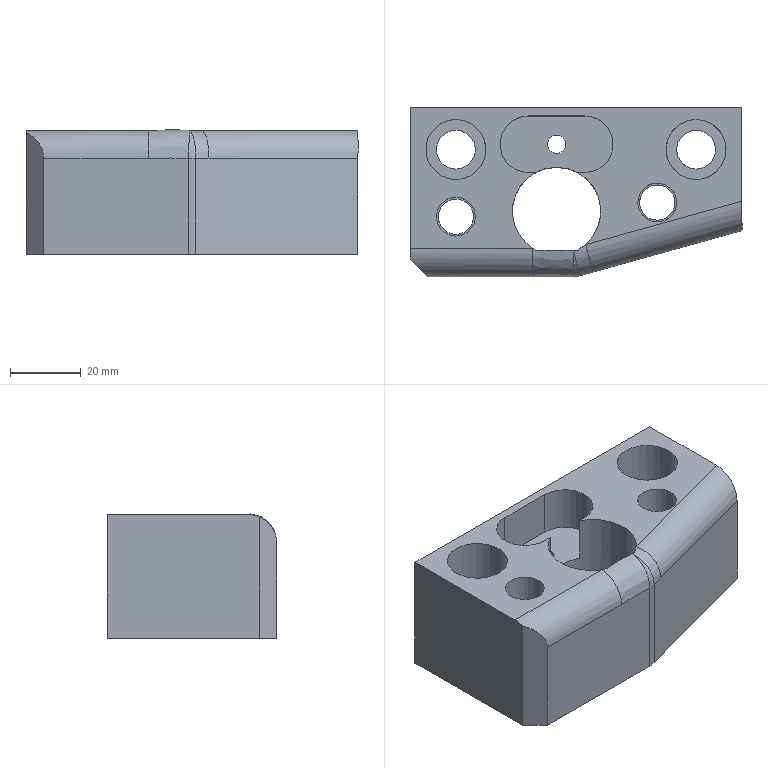Part | STEP file | lll_id4518_x_t | 1 solid | 35 faces | box 94 x 48 x 35.237 mm | volume 104550 mm3 | plane 17 | cylinder 15 | spline 2 | sphere 1 | commonest cylinder face diameters 16 x5 11 x4 10 x2 17 x2 5.206 x1 25 x1
STEP:
#1=CARTESIAN_POINT('',(3581.297,-241.45,-35.));
#2=VERTEX_POINT('',#1);
#3=CARTESIAN_POINT('',(3593.171,-241.45,-35.));
#4=VERTEX_POINT('',#3);
#5=CARTESIAN_POINT('',(3587.234,-230.45,-35.));
#6=DIRECTION('',(0.,0.,-1.));
#7=DIRECTION('',(-1.,0.,0.));
#8=AXIS2_PLACEMENT_3D('',#5,#6,#7);
#9=CIRCLE('',#8,12.5);
#10=EDGE_CURVE('',#2,#4,#9,.T.);
#11=ORIENTED_EDGE('',*,*,#10,.T.);
#12=CARTESIAN_POINT('',(3593.171,-241.45,0.00001673));
#13=VERTEX_POINT('',#12);
#14=CARTESIAN_POINT('',(3593.171,-241.45,-15.));
#15=DIRECTION('',(0.,0.,1.));
#16=VECTOR('',#15,1.);
#17=LINE('',#14,#16);
#18=EDGE_CURVE('',#4,#13,#17,.T.);
#19=ORIENTED_EDGE('',*,*,#18,.T.);
#20=CARTESIAN_POINT('',(3595.413,-239.903,0.00001673));
#21=VERTEX_POINT('',#20);
#22=CARTESIAN_POINT('',(3593.171,-241.45,-0.0001138));
#23=CARTESIAN_POINT('',(3593.485,-241.281,-0.0001498));
#24=CARTESIAN_POINT('',(3593.792,-241.098,-0.0001489));
#25=CARTESIAN_POINT('',(3594.09,-240.902,-0.0001158));
#26=CARTESIAN_POINT('',(3594.552,-240.599,-0.00006449));
#27=CARTESIAN_POINT('',(3594.995,-240.264,0.00001673));
#28=CARTESIAN_POINT('',(3595.413,-239.903,0.00001673));
#29=B_SPLINE_CURVE_WITH_KNOTS('',3,(#22,#23,#24,#25,#26,#27,#28),.UNSPECIFIED.,.F.,.F.,(4,3,4),(0.,0.3921,1.),.UNSPECIFIED.);
#30=EDGE_CURVE('',#13,#21,#29,.T.);
#31=ORIENTED_EDGE('',*,*,#30,.T.);
#32=CARTESIAN_POINT('',(3593.171,-219.45,0.00001673));
#33=VERTEX_POINT('',#32);
#34=CARTESIAN_POINT('',(3587.234,-230.45,0.00001673));
#35=DIRECTION('',(0.,0.,1.));
#36=DIRECTION('',(-1.,0.,0.));
#37=AXIS2_PLACEMENT_3D('',#34,#35,#36);
#38=CIRCLE('',#37,12.5);
#39=EDGE_CURVE('',#21,#33,#38,.T.);
#40=ORIENTED_EDGE('',*,*,#39,.T.);
#41=CARTESIAN_POINT('',(3593.171,-219.45,-13.));
#42=VERTEX_POINT('',#41);
#43=CARTESIAN_POINT('',(3593.171,-219.45,-15.));
#44=DIRECTION('',(0.,0.,1.));
#45=VECTOR('',#44,1.);
#46=LINE('',#43,#45);
#47=EDGE_CURVE('',#42,#33,#46,.T.);
#48=ORIENTED_EDGE('',*,*,#47,.F.);
#49=CARTESIAN_POINT('',(3581.297,-219.45,-13.));
#50=VERTEX_POINT('',#49);
#51=CARTESIAN_POINT('',(3587.234,-230.45,-13.));
#52=DIRECTION('',(0.,0.,1.));
#53=DIRECTION('',(-1.,0.,0.));
#54=AXIS2_PLACEMENT_3D('',#51,#52,#53);
#55=CIRCLE('',#54,12.5);
#56=EDGE_CURVE('',#42,#50,#55,.T.);
#57=ORIENTED_EDGE('',*,*,#56,.T.);
#58=CARTESIAN_POINT('',(3581.297,-219.45,0.00001673));
#59=VERTEX_POINT('',#58);
#60=CARTESIAN_POINT('',(3581.297,-219.45,-15.));
#61=DIRECTION('',(0.,0.,-1.));
#62=VECTOR('',#61,1.);
#63=LINE('',#60,#62);
#64=EDGE_CURVE('',#59,#50,#63,.T.);
#65=ORIENTED_EDGE('',*,*,#64,.F.);
#66=CARTESIAN_POINT('',(3580.452,-240.95,0.00001673));
#67=VERTEX_POINT('',#66);
#68=CARTESIAN_POINT('',(3587.234,-230.45,0.00001673));
#69=DIRECTION('',(0.,0.,1.));
#70=DIRECTION('',(-1.,0.,0.));
#71=AXIS2_PLACEMENT_3D('',#68,#69,#70);
#72=CIRCLE('',#71,12.5);
#73=EDGE_CURVE('',#59,#67,#72,.T.);
#74=ORIENTED_EDGE('',*,*,#73,.T.);
#75=CARTESIAN_POINT('',(3581.297,-241.45,0.00001673));
#76=VERTEX_POINT('',#75);
#77=CARTESIAN_POINT('',(3580.452,-240.95,-0.0008458));
#78=CARTESIAN_POINT('',(3580.727,-241.128,-0.0007971));
#79=CARTESIAN_POINT('',(3581.009,-241.295,-0.0007576));
#80=CARTESIAN_POINT('',(3581.297,-241.45,-0.0007227));
#81=B_SPLINE_CURVE_WITH_KNOTS('',3,(#77,#78,#79,#80),.UNSPECIFIED.,.F.,.F.,(4,4),(0.,1.),.UNSPECIFIED.);
#82=EDGE_CURVE('',#67,#76,#81,.T.);
#83=ORIENTED_EDGE('',*,*,#82,.T.);
#84=CARTESIAN_POINT('',(3581.297,-241.45,-15.));
#85=DIRECTION('',(0.,0.,-1.));
#86=VECTOR('',#85,1.);
#87=LINE('',#84,#86);
#88=EDGE_CURVE('',#76,#2,#87,.T.);
#89=ORIENTED_EDGE('',*,*,#88,.T.);
#90=EDGE_LOOP('',(#11,#19,#31,#40,#48,#57,#65,#74,#83,#89));
#91=FACE_OUTER_BOUND('',#90,.T.);
#92=CARTESIAN_POINT('',(3587.234,-230.45,-15.));
#93=DIRECTION('',(0.,0.,-1.));
#94=DIRECTION('',(1.,0.,0.));
#95=AXIS2_PLACEMENT_3D('',#92,#93,#94);
#96=CYLINDRICAL_SURFACE('',#95,12.5);
#97=ADVANCED_FACE('',(#91),#96,.F.);
#98=CARTESIAN_POINT('',(3618.234,-212.95,0.00001673));
#99=VERTEX_POINT('',#98);
#100=CARTESIAN_POINT('',(3626.734,-212.95,0.00001673));
#101=DIRECTION('',(0.,0.,1.));
#102=DIRECTION('',(-1.,0.,0.));
#103=AXIS2_PLACEMENT_3D('',#100,#101,#102);
#104=CIRCLE('',#103,8.5);
#105=EDGE_CURVE('',#99,#99,#104,.T.);
#106=ORIENTED_EDGE('',*,*,#105,.F.);
#107=EDGE_LOOP('',(#106));
#108=FACE_BOUND('',#107,.T.);
#109=CARTESIAN_POINT('',(3558.734,-226.45,0.00001673));
#110=VERTEX_POINT('',#109);
#111=CARTESIAN_POINT('',(3558.734,-231.95,0.00001673));
#112=DIRECTION('',(0.,0.,1.));
#113=DIRECTION('',(0.,1.,0.));
#114=AXIS2_PLACEMENT_3D('',#111,#112,#113);
#115=CIRCLE('',#114,5.5);
#116=EDGE_CURVE('',#110,#110,#115,.T.);
#117=ORIENTED_EDGE('',*,*,#116,.F.);
#118=EDGE_LOOP('',(#117));
#119=FACE_BOUND('',#118,.T.);
#120=CARTESIAN_POINT('',(3558.734,-221.45,0.00001673));
#121=VERTEX_POINT('',#120);
#122=CARTESIAN_POINT('',(3558.734,-212.95,0.00001673));
#123=DIRECTION('',(0.,0.,-1.));
#124=DIRECTION('',(0.,-1.,0.));
#125=AXIS2_PLACEMENT_3D('',#122,#123,#124);
#126=CIRCLE('',#125,8.5);
#127=EDGE_CURVE('',#121,#121,#126,.T.);
#128=ORIENTED_EDGE('',*,*,#127,.T.);
#129=EDGE_LOOP('',(#128));
#130=FACE_BOUND('',#129,.T.);
#131=CARTESIAN_POINT('',(3610.234,-227.95,0.00001673));
#132=VERTEX_POINT('',#131);
#133=CARTESIAN_POINT('',(3615.734,-227.95,0.00001673));
#134=DIRECTION('',(0.,0.,-1.));
#135=DIRECTION('',(-1.,0.,0.));
#136=AXIS2_PLACEMENT_3D('',#133,#134,#135);
#137=CIRCLE('',#136,5.5);
#138=EDGE_CURVE('',#132,#132,#137,.T.);
#139=ORIENTED_EDGE('',*,*,#138,.T.);
#140=EDGE_LOOP('',(#139));
#141=FACE_BOUND('',#140,.T.);
#142=CARTESIAN_POINT('',(3595.234,-219.45,0.00001673));
#143=VERTEX_POINT('',#142);
#144=CARTESIAN_POINT('',(3595.234,-203.45,0.00001673));
#145=VERTEX_POINT('',#144);
#146=CARTESIAN_POINT('',(3595.234,-211.45,0.00001673));
#147=DIRECTION('',(0.,0.,1.));
#148=DIRECTION('',(1.,0.,0.));
#149=AXIS2_PLACEMENT_3D('',#146,#147,#148);
#150=CIRCLE('',#149,8.);
#151=EDGE_CURVE('',#143,#145,#150,.T.);
#152=ORIENTED_EDGE('',*,*,#151,.F.);
#153=CARTESIAN_POINT('',(3580.234,-219.45,0.00001673));
#154=DIRECTION('',(-1.,0.,0.));
#155=VECTOR('',#154,1.);
#156=LINE('',#153,#155);
#157=EDGE_CURVE('',#143,#33,#156,.T.);
#158=ORIENTED_EDGE('',*,*,#157,.T.);
#159=ORIENTED_EDGE('',*,*,#39,.F.);
#160=CARTESIAN_POINT('',(3639.734,-227.592,0.00001673));
#161=VERTEX_POINT('',#160);
#162=CARTESIAN_POINT('',(3591.947,-240.866,0.00001673));
#163=DIRECTION('',(-0.9635,-0.2676,0.));
#164=VECTOR('',#163,1.);
#165=LINE('',#162,#164);
#166=EDGE_CURVE('',#161,#21,#165,.T.);
#167=ORIENTED_EDGE('',*,*,#166,.F.);
#168=CARTESIAN_POINT('',(3639.734,-200.95,0.00001673));
#169=VERTEX_POINT('',#168);
#170=CARTESIAN_POINT('',(3639.734,-198.7,0.00001673));
#171=DIRECTION('',(0.,-1.,0.));
#172=VECTOR('',#171,1.);
#173=LINE('',#170,#172);
#174=EDGE_CURVE('',#169,#161,#173,.T.);
#175=ORIENTED_EDGE('',*,*,#174,.F.);
#176=CARTESIAN_POINT('',(3545.734,-200.95,0.00001673));
#177=VERTEX_POINT('',#176);
#178=CARTESIAN_POINT('',(3580.234,-200.95,0.00001673));
#179=DIRECTION('',(1.,0.,0.));
#180=VECTOR('',#179,1.);
#181=LINE('',#178,#180);
#182=EDGE_CURVE('',#177,#169,#181,.T.);
#183=ORIENTED_EDGE('',*,*,#182,.F.);
#184=CARTESIAN_POINT('',(3545.734,-240.95,0.00001673));
#185=VERTEX_POINT('',#184);
#186=CARTESIAN_POINT('',(3545.734,-198.7,0.00001673));
#187=DIRECTION('',(0.,1.,0.));
#188=VECTOR('',#187,1.);
#189=LINE('',#186,#188);
#190=EDGE_CURVE('',#185,#177,#189,.T.);
#191=ORIENTED_EDGE('',*,*,#190,.F.);
#192=CARTESIAN_POINT('',(3580.234,-240.95,0.00001673));
#193=DIRECTION('',(-1.,0.,0.));
#194=VECTOR('',#193,1.);
#195=LINE('',#192,#194);
#196=EDGE_CURVE('',#67,#185,#195,.T.);
#197=ORIENTED_EDGE('',*,*,#196,.F.);
#198=ORIENTED_EDGE('',*,*,#73,.F.);
#199=CARTESIAN_POINT('',(3579.234,-219.45,0.00001673));
#200=VERTEX_POINT('',#199);
#201=CARTESIAN_POINT('',(3580.234,-219.45,0.00001673));
#202=DIRECTION('',(-1.,0.,0.));
#203=VECTOR('',#202,1.);
#204=LINE('',#201,#203);
#205=EDGE_CURVE('',#59,#200,#204,.T.);
#206=ORIENTED_EDGE('',*,*,#205,.T.);
#207=CARTESIAN_POINT('',(3579.234,-203.45,0.00001673));
#208=VERTEX_POINT('',#207);
#209=CARTESIAN_POINT('',(3579.234,-211.45,0.00001673));
#210=DIRECTION('',(0.,0.,1.));
#211=DIRECTION('',(1.,0.,0.));
#212=AXIS2_PLACEMENT_3D('',#209,#210,#211);
#213=CIRCLE('',#212,8.);
#214=EDGE_CURVE('',#208,#200,#213,.T.);
#215=ORIENTED_EDGE('',*,*,#214,.F.);
#216=CARTESIAN_POINT('',(3580.234,-203.45,0.00001673));
#217=DIRECTION('',(-1.,0.,0.));
#218=VECTOR('',#217,1.);
#219=LINE('',#216,#218);
#220=EDGE_CURVE('',#145,#208,#219,.T.);
#221=ORIENTED_EDGE('',*,*,#220,.F.);
#222=EDGE_LOOP('',(#152,#158,#159,#167,#175,#183,#191,#197,#198,#206,#215,#221));
#223=FACE_BOUND('',#222,.T.);
#224=CARTESIAN_POINT('',(3580.234,-198.7,0.00001673));
#225=DIRECTION('',(0.,0.,1.));
#226=DIRECTION('',(0.,1.,0.));
#227=AXIS2_PLACEMENT_3D('',#224,#225,#226);
#228=PLANE('',#227);
#229=ADVANCED_FACE('',(#108,#119,#130,#141,#223),#228,.T.);
#230=CARTESIAN_POINT('',(3558.734,-218.45,-20.));
#231=VERTEX_POINT('',#230);
#232=CARTESIAN_POINT('',(3558.734,-212.95,-20.));
#233=DIRECTION('',(0.,0.,-1.));
#234=DIRECTION('',(0.,-1.,0.));
#235=AXIS2_PLACEMENT_3D('',#232,#233,#234);
#236=CIRCLE('',#235,5.5);
#237=EDGE_CURVE('',#231,#231,#236,.T.);
#238=ORIENTED_EDGE('',*,*,#237,.T.);
#239=EDGE_LOOP('',(#238));
#240=FACE_BOUND('',#239,.T.);
#241=CARTESIAN_POINT('',(3558.734,-204.45,-20.));
#242=VERTEX_POINT('',#241);
#243=CARTESIAN_POINT('',(3558.734,-212.95,-20.));
#244=DIRECTION('',(0.,0.,1.));
#245=DIRECTION('',(0.,1.,0.));
#246=AXIS2_PLACEMENT_3D('',#243,#244,#245);
#247=CIRCLE('',#246,8.5);
#248=EDGE_CURVE('',#242,#242,#247,.T.);
#249=ORIENTED_EDGE('',*,*,#248,.T.);
#250=EDGE_LOOP('',(#249));
#251=FACE_BOUND('',#250,.T.);
#252=CARTESIAN_POINT('',(3558.734,-212.95,-20.));
#253=DIRECTION('',(0.,0.,-1.));
#254=DIRECTION('',(0.,-1.,0.));
#255=AXIS2_PLACEMENT_3D('',#252,#253,#254);
#256=PLANE('',#255);
#257=ADVANCED_FACE('',(#240,#251),#256,.F.);
#258=CARTESIAN_POINT('',(3558.734,-226.45,-15.));
#259=VERTEX_POINT('',#258);
#260=CARTESIAN_POINT('',(3558.734,-231.95,-15.));
#261=DIRECTION('',(0.,0.,1.));
#262=DIRECTION('',(0.,1.,0.));
#263=AXIS2_PLACEMENT_3D('',#260,#261,#262);
#264=CIRCLE('',#263,5.5);
#265=EDGE_CURVE('',#259,#259,#264,.T.);
#266=ORIENTED_EDGE('',*,*,#265,.T.);
#267=EDGE_LOOP('',(#266));
#268=FACE_BOUND('',#267,.T.);
#269=CARTESIAN_POINT('',(3558.734,-226.95,-15.));
#270=VERTEX_POINT('',#269);
#271=CARTESIAN_POINT('',(3558.734,-231.95,-15.));
#272=DIRECTION('',(0.,0.,1.));
#273=DIRECTION('',(0.,1.,0.));
#274=AXIS2_PLACEMENT_3D('',#271,#272,#273);
#275=CIRCLE('',#274,5.);
#276=EDGE_CURVE('',#270,#270,#275,.T.);
#277=ORIENTED_EDGE('',*,*,#276,.F.);
#278=EDGE_LOOP('',(#277));
#279=FACE_BOUND('',#278,.T.);
#280=CARTESIAN_POINT('',(3558.734,-231.95,-15.));
#281=DIRECTION('',(0.,0.,-1.));
#282=DIRECTION('',(0.,1.,0.));
#283=AXIS2_PLACEMENT_3D('',#280,#281,#282);
#284=PLANE('',#283);
#285=ADVANCED_FACE('',(#268,#279),#284,.F.);
#286=CARTESIAN_POINT('',(3558.734,-207.45,-35.));
#287=VERTEX_POINT('',#286);
#288=CARTESIAN_POINT('',(3558.734,-212.95,-35.));
#289=DIRECTION('',(0.,0.,1.));
#290=DIRECTION('',(0.,1.,0.));
#291=AXIS2_PLACEMENT_3D('',#288,#289,#290);
#292=CIRCLE('',#291,5.5);
#293=EDGE_CURVE('',#287,#287,#292,.T.);
#294=ORIENTED_EDGE('',*,*,#293,.F.);
#295=EDGE_LOOP('',(#294));
#296=FACE_BOUND('',#295,.T.);
#297=ORIENTED_EDGE('',*,*,#237,.F.);
#298=EDGE_LOOP('',(#297));
#299=FACE_BOUND('',#298,.T.);
#300=CARTESIAN_POINT('',(3558.734,-212.95,-20.));
#301=DIRECTION('',(0.,0.,-1.));
#302=DIRECTION('',(0.,-1.,0.));
#303=AXIS2_PLACEMENT_3D('',#300,#301,#302);
#304=CYLINDRICAL_SURFACE('',#303,5.5);
#305=ADVANCED_FACE('',(#296,#299),#304,.F.);
#306=CARTESIAN_POINT('',(3639.734,-200.95,-35.));
#307=VERTEX_POINT('',#306);
#308=CARTESIAN_POINT('',(3545.734,-200.95,-35.));
#309=VERTEX_POINT('',#308);
#310=CARTESIAN_POINT('',(3580.234,-200.95,-35.));
#311=DIRECTION('',(-1.,0.,0.));
#312=VECTOR('',#311,1.);
#313=LINE('',#310,#312);
#314=EDGE_CURVE('',#307,#309,#313,.T.);
#315=ORIENTED_EDGE('',*,*,#314,.T.);
#316=CARTESIAN_POINT('',(3545.734,-200.95,-65.));
#317=DIRECTION('',(0.,0.,-1.));
#318=VECTOR('',#317,1.);
#319=LINE('',#316,#318);
#320=EDGE_CURVE('',#177,#309,#319,.T.);
#321=ORIENTED_EDGE('',*,*,#320,.F.);
#322=ORIENTED_EDGE('',*,*,#182,.T.);
#323=CARTESIAN_POINT('',(3639.734,-200.95,-65.));
#324=DIRECTION('',(0.,0.,-1.));
#325=VECTOR('',#324,1.);
#326=LINE('',#323,#325);
#327=EDGE_CURVE('',#169,#307,#326,.T.);
#328=ORIENTED_EDGE('',*,*,#327,.T.);
#329=EDGE_LOOP('',(#315,#321,#322,#328));
#330=FACE_OUTER_BOUND('',#329,.T.);
#331=CARTESIAN_POINT('',(3580.234,-200.95,-65.));
#332=DIRECTION('',(0.,1.,0.));
#333=DIRECTION('',(0.,0.,-1.));
#334=AXIS2_PLACEMENT_3D('',#331,#332,#333);
#335=PLANE('',#334);
#336=ADVANCED_FACE('',(#330),#335,.T.);
#337=CARTESIAN_POINT('',(3639.734,-235.894,-35.));
#338=VERTEX_POINT('',#337);
#339=CARTESIAN_POINT('',(3639.734,-235.894,-8.));
#340=VERTEX_POINT('',#339);
#341=CARTESIAN_POINT('',(3639.734,-235.894,-65.));
#342=DIRECTION('',(0.,0.,1.));
#343=VECTOR('',#342,1.);
#344=LINE('',#341,#343);
#345=EDGE_CURVE('',#338,#340,#344,.T.);
#346=ORIENTED_EDGE('',*,*,#345,.F.);
#347=CARTESIAN_POINT('',(3639.734,-198.7,-35.));
#348=DIRECTION('',(0.,1.,0.));
#349=VECTOR('',#348,1.);
#350=LINE('',#347,#349);
#351=EDGE_CURVE('',#338,#307,#350,.T.);
#352=ORIENTED_EDGE('',*,*,#351,.T.);
#353=ORIENTED_EDGE('',*,*,#327,.F.);
#354=ORIENTED_EDGE('',*,*,#174,.T.);
#355=CARTESIAN_POINT('',(3639.734,-227.592,-8.));
#356=DIRECTION('',(-1.,0.,0.));
#357=DIRECTION('',(0.,1.,0.));
#358=AXIS2_PLACEMENT_3D('',#355,#356,#357);
#359=ELLIPSE('',#358,8.303,8.);
#360=EDGE_CURVE('',#340,#161,#359,.T.);
#361=ORIENTED_EDGE('',*,*,#360,.F.);
#362=EDGE_LOOP('',(#346,#352,#353,#354,#361));
#363=FACE_OUTER_BOUND('',#362,.T.);
#364=CARTESIAN_POINT('',(3639.734,-198.7,-65.));
#365=DIRECTION('',(1.,0.,0.));
#366=DIRECTION('',(0.,0.,-1.));
#367=AXIS2_PLACEMENT_3D('',#364,#365,#366);
#368=PLANE('',#367);
#369=ADVANCED_FACE('',(#363),#368,.T.);
#370=CARTESIAN_POINT('',(3550.734,-248.95,-35.));
#371=VERTEX_POINT('',#370);
#372=CARTESIAN_POINT('',(3591.644,-248.95,-35.));
#373=VERTEX_POINT('',#372);
#374=CARTESIAN_POINT('',(3580.234,-248.95,-35.));
#375=DIRECTION('',(1.,0.,0.));
#376=VECTOR('',#375,1.);
#377=LINE('',#374,#376);
#378=EDGE_CURVE('',#371,#373,#377,.T.);
#379=ORIENTED_EDGE('',*,*,#378,.T.);
#380=CARTESIAN_POINT('',(3591.644,-248.95,-7.922));
#381=VERTEX_POINT('',#380);
#382=CARTESIAN_POINT('',(3591.644,-248.95,-65.));
#383=DIRECTION('',(0.,0.,-1.));
#384=VECTOR('',#383,1.);
#385=LINE('',#382,#384);
#386=EDGE_CURVE('',#381,#373,#385,.T.);
#387=ORIENTED_EDGE('',*,*,#386,.F.);
#388=CARTESIAN_POINT('',(3580.452,-248.95,-8.));
#389=VERTEX_POINT('',#388);
#390=CARTESIAN_POINT('',(3580.452,-248.95,-8.));
#391=CARTESIAN_POINT('',(3582.321,-248.95,-8.));
#392=CARTESIAN_POINT('',(3584.183,-248.95,-7.815));
#393=CARTESIAN_POINT('',(3587.918,-248.95,-7.711));
#394=CARTESIAN_POINT('',(3589.781,-248.95,-7.821));
#395=CARTESIAN_POINT('',(3591.644,-248.95,-7.922));
#396=B_SPLINE_CURVE_WITH_KNOTS('',3,(#390,#391,#392,#393,#394,#395),.UNSPECIFIED.,.F.,.F.,(4,2,4),(0.,0.5,1.),.UNSPECIFIED.);
#397=EDGE_CURVE('',#389,#381,#396,.T.);
#398=ORIENTED_EDGE('',*,*,#397,.F.);
#399=CARTESIAN_POINT('',(3550.734,-248.95,-8.));
#400=VERTEX_POINT('',#399);
#401=CARTESIAN_POINT('',(3580.234,-248.95,-8.));
#402=DIRECTION('',(1.,0.,0.));
#403=VECTOR('',#402,1.);
#404=LINE('',#401,#403);
#405=EDGE_CURVE('',#400,#389,#404,.T.);
#406=ORIENTED_EDGE('',*,*,#405,.F.);
#407=CARTESIAN_POINT('',(3550.734,-248.95,-65.));
#408=DIRECTION('',(0.,0.,1.));
#409=VECTOR('',#408,1.);
#410=LINE('',#407,#409);
#411=EDGE_CURVE('',#371,#400,#410,.T.);
#412=ORIENTED_EDGE('',*,*,#411,.F.);
#413=EDGE_LOOP('',(#379,#387,#398,#406,#412));
#414=FACE_OUTER_BOUND('',#413,.T.);
#415=CARTESIAN_POINT('',(3580.234,-248.95,-65.));
#416=DIRECTION('',(0.,-1.,0.));
#417=DIRECTION('',(0.,0.,1.));
#418=AXIS2_PLACEMENT_3D('',#415,#416,#417);
#419=PLANE('',#418);
#420=ADVANCED_FACE('',(#414),#419,.T.);
#421=CARTESIAN_POINT('',(3545.734,-243.95,-0.5838));
#422=VERTEX_POINT('',#421);
#423=CARTESIAN_POINT('',(3545.734,-240.95,-8.));
#424=DIRECTION('',(1.,0.,0.));
#425=DIRECTION('',(0.,0.,-1.));
#426=AXIS2_PLACEMENT_3D('',#423,#424,#425);
#427=CIRCLE('',#426,8.);
#428=EDGE_CURVE('',#185,#422,#427,.T.);
#429=ORIENTED_EDGE('',*,*,#428,.F.);
#430=ORIENTED_EDGE('',*,*,#190,.T.);
#431=ORIENTED_EDGE('',*,*,#320,.T.);
#432=CARTESIAN_POINT('',(3545.734,-243.95,-35.));
#433=VERTEX_POINT('',#432);
#434=CARTESIAN_POINT('',(3545.734,-198.7,-35.));
#435=DIRECTION('',(0.,-1.,0.));
#436=VECTOR('',#435,1.);
#437=LINE('',#434,#436);
#438=EDGE_CURVE('',#309,#433,#437,.T.);
#439=ORIENTED_EDGE('',*,*,#438,.T.);
#440=CARTESIAN_POINT('',(3545.734,-243.95,-65.));
#441=DIRECTION('',(0.,0.,-1.));
#442=VECTOR('',#441,1.);
#443=LINE('',#440,#442);
#444=EDGE_CURVE('',#422,#433,#443,.T.);
#445=ORIENTED_EDGE('',*,*,#444,.F.);
#446=EDGE_LOOP('',(#429,#430,#431,#439,#445));
#447=FACE_OUTER_BOUND('',#446,.T.);
#448=CARTESIAN_POINT('',(3545.734,-198.7,-65.));
#449=DIRECTION('',(-1.,0.,0.));
#450=DIRECTION('',(0.,0.,1.));
#451=AXIS2_PLACEMENT_3D('',#448,#449,#450);
#452=PLANE('',#451);
#453=ADVANCED_FACE('',(#447),#452,.T.);
#454=ORIENTED_EDGE('',*,*,#276,.T.);
#455=EDGE_LOOP('',(#454));
#456=FACE_BOUND('',#455,.T.);
#457=CARTESIAN_POINT('',(3558.734,-236.95,-35.));
#458=VERTEX_POINT('',#457);
#459=CARTESIAN_POINT('',(3558.734,-231.95,-35.));
#460=DIRECTION('',(0.,0.,1.));
#461=DIRECTION('',(0.,-1.,0.));
#462=AXIS2_PLACEMENT_3D('',#459,#460,#461);
#463=CIRCLE('',#462,5.);
#464=EDGE_CURVE('',#458,#458,#463,.T.);
#465=ORIENTED_EDGE('',*,*,#464,.F.);
#466=EDGE_LOOP('',(#465));
#467=FACE_BOUND('',#466,.T.);
#468=CARTESIAN_POINT('',(3558.734,-231.95,-20.));
#469=DIRECTION('',(0.,0.,-1.));
#470=DIRECTION('',(0.,1.,0.));
#471=AXIS2_PLACEMENT_3D('',#468,#469,#470);
#472=CYLINDRICAL_SURFACE('',#471,5.);
#473=ADVANCED_FACE('',(#456,#467),#472,.F.);
#474=CARTESIAN_POINT('',(3584.631,-211.45,-35.));
#475=VERTEX_POINT('',#474);
#476=CARTESIAN_POINT('',(3587.234,-211.45,-35.));
#477=DIRECTION('',(0.,0.,-1.));
#478=DIRECTION('',(-1.,0.,0.));
#479=AXIS2_PLACEMENT_3D('',#476,#477,#478);
#480=CIRCLE('',#479,2.603);
#481=EDGE_CURVE('',#475,#475,#480,.T.);
#482=ORIENTED_EDGE('',*,*,#481,.F.);
#483=EDGE_LOOP('',(#482));
#484=FACE_BOUND('',#483,.T.);
#485=ORIENTED_EDGE('',*,*,#10,.F.);
#486=CARTESIAN_POINT('',(3587.234,-241.45,-35.));
#487=DIRECTION('',(1.,0.,0.));
#488=VECTOR('',#487,1.);
#489=LINE('',#486,#488);
#490=EDGE_CURVE('',#2,#4,#489,.T.);
#491=ORIENTED_EDGE('',*,*,#490,.T.);
#492=EDGE_LOOP('',(#485,#491));
#493=FACE_BOUND('',#492,.T.);
#494=CARTESIAN_POINT('',(3632.234,-212.95,-35.));
#495=VERTEX_POINT('',#494);
#496=CARTESIAN_POINT('',(3626.734,-212.95,-35.));
#497=DIRECTION('',(0.,0.,1.));
#498=DIRECTION('',(1.,0.,0.));
#499=AXIS2_PLACEMENT_3D('',#496,#497,#498);
#500=CIRCLE('',#499,5.5);
#501=EDGE_CURVE('',#495,#495,#500,.T.);
#502=ORIENTED_EDGE('',*,*,#501,.T.);
#503=EDGE_LOOP('',(#502));
#504=FACE_BOUND('',#503,.T.);
#505=CARTESIAN_POINT('',(3620.734,-227.95,-35.));
#506=VERTEX_POINT('',#505);
#507=CARTESIAN_POINT('',(3615.734,-227.95,-35.));
#508=DIRECTION('',(0.,0.,1.));
#509=DIRECTION('',(1.,0.,0.));
#510=AXIS2_PLACEMENT_3D('',#507,#508,#509);
#511=CIRCLE('',#510,5.);
#512=EDGE_CURVE('',#506,#506,#511,.T.);
#513=ORIENTED_EDGE('',*,*,#512,.T.);
#514=EDGE_LOOP('',(#513));
#515=FACE_BOUND('',#514,.T.);
#516=ORIENTED_EDGE('',*,*,#464,.T.);
#517=EDGE_LOOP('',(#516));
#518=FACE_BOUND('',#517,.T.);
#519=ORIENTED_EDGE('',*,*,#438,.F.);
#520=ORIENTED_EDGE('',*,*,#314,.F.);
#521=ORIENTED_EDGE('',*,*,#351,.F.);
#522=CARTESIAN_POINT('',(3593.785,-248.658,-35.));
#523=VERTEX_POINT('',#522);
#524=CARTESIAN_POINT('',(3594.088,-248.574,-35.));
#525=DIRECTION('',(0.9635,0.2676,0.));
#526=VECTOR('',#525,1.);
#527=LINE('',#524,#526);
#528=EDGE_CURVE('',#523,#338,#527,.T.);
#529=ORIENTED_EDGE('',*,*,#528,.F.);
#530=CARTESIAN_POINT('',(3591.644,-240.95,-35.));
#531=DIRECTION('',(0.,0.,1.));
#532=DIRECTION('',(1.,0.,0.));
#533=AXIS2_PLACEMENT_3D('',#530,#531,#532);
#534=CIRCLE('',#533,8.);
#535=EDGE_CURVE('',#373,#523,#534,.T.);
#536=ORIENTED_EDGE('',*,*,#535,.F.);
#537=ORIENTED_EDGE('',*,*,#378,.F.);
#538=CARTESIAN_POINT('',(3540.359,-238.575,-35.));
#539=DIRECTION('',(0.7071,-0.7071,0.));
#540=VECTOR('',#539,1.);
#541=LINE('',#538,#540);
#542=EDGE_CURVE('',#433,#371,#541,.T.);
#543=ORIENTED_EDGE('',*,*,#542,.F.);
#544=EDGE_LOOP('',(#519,#520,#521,#529,#536,#537,#543));
#545=FACE_BOUND('',#544,.T.);
#546=ORIENTED_EDGE('',*,*,#293,.T.);
#547=EDGE_LOOP('',(#546));
#548=FACE_BOUND('',#547,.T.);
#549=CARTESIAN_POINT('',(3580.234,-198.7,-35.));
#550=DIRECTION('',(0.,0.,-1.));
#551=DIRECTION('',(0.,-1.,0.));
#552=AXIS2_PLACEMENT_3D('',#549,#550,#551);
#553=PLANE('',#552);
#554=ADVANCED_FACE('',(#484,#493,#504,#515,#518,#545,#548),#553,.T.);
#555=ORIENTED_EDGE('',*,*,#265,.F.);
#556=EDGE_LOOP('',(#555));
#557=FACE_BOUND('',#556,.T.);
#558=ORIENTED_EDGE('',*,*,#116,.T.);
#559=EDGE_LOOP('',(#558));
#560=FACE_BOUND('',#559,.T.);
#561=CARTESIAN_POINT('',(3558.734,-231.95,0.00001673));
#562=DIRECTION('',(0.,0.,-1.));
#563=DIRECTION('',(0.,1.,0.));
#564=AXIS2_PLACEMENT_3D('',#561,#562,#563);
#565=CYLINDRICAL_SURFACE('',#564,5.5);
#566=ADVANCED_FACE('',(#557,#560),#565,.F.);
#567=ORIENTED_EDGE('',*,*,#248,.F.);
#568=EDGE_LOOP('',(#567));
#569=FACE_BOUND('',#568,.T.);
#570=ORIENTED_EDGE('',*,*,#127,.F.);
#571=EDGE_LOOP('',(#570));
#572=FACE_BOUND('',#571,.T.);
#573=CARTESIAN_POINT('',(3558.734,-212.95,-20.));
#574=DIRECTION('',(0.,0.,1.));
#575=DIRECTION('',(0.,1.,0.));
#576=AXIS2_PLACEMENT_3D('',#573,#574,#575);
#577=CYLINDRICAL_SURFACE('',#576,8.5);
#578=ADVANCED_FACE('',(#569,#572),#577,.F.);
#579=CARTESIAN_POINT('',(3615.734,-222.45,-15.));
#580=VERTEX_POINT('',#579);
#581=CARTESIAN_POINT('',(3615.734,-227.95,-15.));
#582=DIRECTION('',(0.,0.,1.));
#583=DIRECTION('',(0.,1.,0.));
#584=AXIS2_PLACEMENT_3D('',#581,#582,#583);
#585=CIRCLE('',#584,5.5);
#586=EDGE_CURVE('',#580,#580,#585,.T.);
#587=ORIENTED_EDGE('',*,*,#586,.T.);
#588=EDGE_LOOP('',(#587));
#589=FACE_BOUND('',#588,.T.);
#590=CARTESIAN_POINT('',(3615.734,-222.95,-15.));
#591=VERTEX_POINT('',#590);
#592=CARTESIAN_POINT('',(3615.734,-227.95,-15.));
#593=DIRECTION('',(0.,0.,1.));
#594=DIRECTION('',(0.,1.,0.));
#595=AXIS2_PLACEMENT_3D('',#592,#593,#594);
#596=CIRCLE('',#595,5.);
#597=EDGE_CURVE('',#591,#591,#596,.T.);
#598=ORIENTED_EDGE('',*,*,#597,.F.);
#599=EDGE_LOOP('',(#598));
#600=FACE_BOUND('',#599,.T.);
#601=CARTESIAN_POINT('',(3615.734,-227.95,-15.));
#602=DIRECTION('',(0.,0.,-1.));
#603=DIRECTION('',(0.,1.,0.));
#604=AXIS2_PLACEMENT_3D('',#601,#602,#603);
#605=PLANE('',#604);
#606=ADVANCED_FACE('',(#589,#600),#605,.F.);
#607=ORIENTED_EDGE('',*,*,#597,.T.);
#608=EDGE_LOOP('',(#607));
#609=FACE_BOUND('',#608,.T.);
#610=ORIENTED_EDGE('',*,*,#512,.F.);
#611=EDGE_LOOP('',(#610));
#612=FACE_BOUND('',#611,.T.);
#613=CARTESIAN_POINT('',(3615.734,-227.95,-20.));
#614=DIRECTION('',(0.,0.,-1.));
#615=DIRECTION('',(0.,1.,0.));
#616=AXIS2_PLACEMENT_3D('',#613,#614,#615);
#617=CYLINDRICAL_SURFACE('',#616,5.);
#618=ADVANCED_FACE('',(#609,#612),#617,.F.);
#619=ORIENTED_EDGE('',*,*,#586,.F.);
#620=EDGE_LOOP('',(#619));
#621=FACE_BOUND('',#620,.T.);
#622=ORIENTED_EDGE('',*,*,#138,.F.);
#623=EDGE_LOOP('',(#622));
#624=FACE_BOUND('',#623,.T.);
#625=CARTESIAN_POINT('',(3615.734,-227.95,0.00001673));
#626=DIRECTION('',(0.,0.,-1.));
#627=DIRECTION('',(0.,1.,0.));
#628=AXIS2_PLACEMENT_3D('',#625,#626,#627);
#629=CYLINDRICAL_SURFACE('',#628,5.5);
#630=ADVANCED_FACE('',(#621,#624),#629,.F.);
#631=CARTESIAN_POINT('',(3626.734,-218.45,-20.));
#632=VERTEX_POINT('',#631);
#633=CARTESIAN_POINT('',(3626.734,-212.95,-20.));
#634=DIRECTION('',(0.,0.,-1.));
#635=DIRECTION('',(0.,-1.,0.));
#636=AXIS2_PLACEMENT_3D('',#633,#634,#635);
#637=CIRCLE('',#636,5.5);
#638=EDGE_CURVE('',#632,#632,#637,.T.);
#639=ORIENTED_EDGE('',*,*,#638,.T.);
#640=EDGE_LOOP('',(#639));
#641=FACE_BOUND('',#640,.T.);
#642=CARTESIAN_POINT('',(3626.734,-204.45,-20.));
#643=VERTEX_POINT('',#642);
#644=CARTESIAN_POINT('',(3626.734,-212.95,-20.));
#645=DIRECTION('',(0.,0.,1.));
#646=DIRECTION('',(0.,1.,0.));
#647=AXIS2_PLACEMENT_3D('',#644,#645,#646);
#648=CIRCLE('',#647,8.5);
#649=EDGE_CURVE('',#643,#643,#648,.T.);
#650=ORIENTED_EDGE('',*,*,#649,.T.);
#651=EDGE_LOOP('',(#650));
#652=FACE_BOUND('',#651,.T.);
#653=CARTESIAN_POINT('',(3626.734,-212.95,-20.));
#654=DIRECTION('',(0.,0.,-1.));
#655=DIRECTION('',(0.,-1.,0.));
#656=AXIS2_PLACEMENT_3D('',#653,#654,#655);
#657=PLANE('',#656);
#658=ADVANCED_FACE('',(#641,#652),#657,.F.);
#659=ORIENTED_EDGE('',*,*,#501,.F.);
#660=EDGE_LOOP('',(#659));
#661=FACE_BOUND('',#660,.T.);
#662=ORIENTED_EDGE('',*,*,#638,.F.);
#663=EDGE_LOOP('',(#662));
#664=FACE_BOUND('',#663,.T.);
#665=CARTESIAN_POINT('',(3626.734,-212.95,-20.));
#666=DIRECTION('',(0.,0.,-1.));
#667=DIRECTION('',(0.,-1.,0.));
#668=AXIS2_PLACEMENT_3D('',#665,#666,#667);
#669=CYLINDRICAL_SURFACE('',#668,5.5);
#670=ADVANCED_FACE('',(#661,#664),#669,.F.);
#671=ORIENTED_EDGE('',*,*,#649,.F.);
#672=EDGE_LOOP('',(#671));
#673=FACE_BOUND('',#672,.T.);
#674=ORIENTED_EDGE('',*,*,#105,.T.);
#675=EDGE_LOOP('',(#674));
#676=FACE_BOUND('',#675,.T.);
#677=CARTESIAN_POINT('',(3626.734,-212.95,-20.));
#678=DIRECTION('',(0.,0.,1.));
#679=DIRECTION('',(0.,1.,0.));
#680=AXIS2_PLACEMENT_3D('',#677,#678,#679);
#681=CYLINDRICAL_SURFACE('',#680,8.5);
#682=ADVANCED_FACE('',(#673,#676),#681,.F.);
#683=CARTESIAN_POINT('',(3593.785,-248.658,-7.922));
#684=VERTEX_POINT('',#683);
#685=CARTESIAN_POINT('',(3593.785,-248.658,-65.));
#686=DIRECTION('',(0.,0.,1.));
#687=VECTOR('',#686,1.);
#688=LINE('',#685,#687);
#689=EDGE_CURVE('',#523,#684,#688,.T.);
#690=ORIENTED_EDGE('',*,*,#689,.F.);
#691=ORIENTED_EDGE('',*,*,#528,.T.);
#692=ORIENTED_EDGE('',*,*,#345,.T.);
#693=CARTESIAN_POINT('',(3597.554,-247.611,-8.));
#694=VERTEX_POINT('',#693);
#695=CARTESIAN_POINT('',(3592.734,-248.95,-8.));
#696=DIRECTION('',(0.9635,0.2676,0.));
#697=VECTOR('',#696,1.);
#698=LINE('',#695,#697);
#699=EDGE_CURVE('',#694,#340,#698,.T.);
#700=ORIENTED_EDGE('',*,*,#699,.F.);
#701=CARTESIAN_POINT('',(3593.785,-248.658,-7.922));
#702=CARTESIAN_POINT('',(3594.503,-248.459,-7.936));
#703=CARTESIAN_POINT('',(3595.222,-248.259,-7.958));
#704=CARTESIAN_POINT('',(3596.478,-247.91,-7.989));
#705=CARTESIAN_POINT('',(3597.016,-247.761,-8.));
#706=CARTESIAN_POINT('',(3597.554,-247.611,-8.));
#707=B_SPLINE_CURVE_WITH_KNOTS('',3,(#701,#702,#703,#704,#705,#706),.UNSPECIFIED.,.F.,.F.,(4,2,4),(0.,0.572,1.),.UNSPECIFIED.);
#708=EDGE_CURVE('',#684,#694,#707,.T.);
#709=ORIENTED_EDGE('',*,*,#708,.F.);
#710=EDGE_LOOP('',(#690,#691,#692,#700,#709));
#711=FACE_OUTER_BOUND('',#710,.T.);
#712=CARTESIAN_POINT('',(3592.734,-248.95,-65.));
#713=DIRECTION('',(-0.2676,0.9635,0.));
#714=DIRECTION('',(0.,0.,-1.));
#715=AXIS2_PLACEMENT_3D('',#712,#713,#714);
#716=PLANE('',#715);
#717=ADVANCED_FACE('',(#711),#716,.F.);
#718=ORIENTED_EDGE('',*,*,#386,.T.);
#719=ORIENTED_EDGE('',*,*,#535,.T.);
#720=ORIENTED_EDGE('',*,*,#689,.T.);
#721=CARTESIAN_POINT('',(3591.644,-240.95,-7.922));
#722=DIRECTION('',(0.,0.,1.));
#723=DIRECTION('',(-1.,0.,0.));
#724=AXIS2_PLACEMENT_3D('',#721,#722,#723);
#725=CIRCLE('',#724,8.);
#726=EDGE_CURVE('',#381,#684,#725,.T.);
#727=ORIENTED_EDGE('',*,*,#726,.F.);
#728=EDGE_LOOP('',(#718,#719,#720,#727));
#729=FACE_OUTER_BOUND('',#728,.T.);
#730=CARTESIAN_POINT('',(3591.644,-240.95,-65.));
#731=DIRECTION('',(0.,0.,1.));
#732=DIRECTION('',(-1.,0.,0.));
#733=AXIS2_PLACEMENT_3D('',#730,#731,#732);
#734=CYLINDRICAL_SURFACE('',#733,8.);
#735=ADVANCED_FACE('',(#729),#734,.T.);
#736=ORIENTED_EDGE('',*,*,#360,.T.);
#737=ORIENTED_EDGE('',*,*,#166,.T.);
#738=CARTESIAN_POINT('',(3595.413,-239.903,-8.));
#739=DIRECTION('',(0.9635,0.2676,0.));
#740=DIRECTION('',(-0.2676,0.9635,0.));
#741=AXIS2_PLACEMENT_3D('',#738,#739,#740);
#742=CIRCLE('',#741,8.);
#743=EDGE_CURVE('',#21,#694,#742,.T.);
#744=ORIENTED_EDGE('',*,*,#743,.T.);
#745=ORIENTED_EDGE('',*,*,#699,.T.);
#746=EDGE_LOOP('',(#736,#737,#744,#745));
#747=FACE_OUTER_BOUND('',#746,.T.);
#748=CARTESIAN_POINT('',(3591.947,-240.866,-8.));
#749=DIRECTION('',(0.9635,0.2676,0.));
#750=DIRECTION('',(0.2676,-0.9635,0.));
#751=AXIS2_PLACEMENT_3D('',#748,#749,#750);
#752=CYLINDRICAL_SURFACE('',#751,8.);
#753=ADVANCED_FACE('',(#747),#752,.T.);
#754=ORIENTED_EDGE('',*,*,#743,.F.);
#755=ORIENTED_EDGE('',*,*,#30,.F.);
#756=CARTESIAN_POINT('',(3592.074,-241.975,0.00001673));
#757=VERTEX_POINT('',#756);
#758=CARTESIAN_POINT('',(3592.074,-241.975,-0.0006541));
#759=CARTESIAN_POINT('',(3592.465,-241.811,-0.0006607));
#760=CARTESIAN_POINT('',(3592.831,-241.634,-0.0006801));
#761=CARTESIAN_POINT('',(3593.171,-241.45,-0.0007151));
#762=B_SPLINE_CURVE_WITH_KNOTS('',3,(#758,#759,#760,#761),.UNSPECIFIED.,.F.,.F.,(4,4),(0.,1.),.UNSPECIFIED.);
#763=EDGE_CURVE('',#757,#13,#762,.T.);
#764=ORIENTED_EDGE('',*,*,#763,.F.);
#765=CARTESIAN_POINT('',(3591.644,-240.95,-7.922));
#766=DIRECTION('',(0.9634,0.2676,-0.01772));
#767=DIRECTION('',(-0.2676,0.9635,0.));
#768=AXIS2_PLACEMENT_3D('',#765,#766,#767);
#769=CIRCLE('',#768,8.);
#770=EDGE_CURVE('',#757,#684,#769,.T.);
#771=ORIENTED_EDGE('',*,*,#770,.T.);
#772=ORIENTED_EDGE('',*,*,#708,.T.);
#773=EDGE_LOOP('',(#754,#755,#764,#771,#772));
#774=FACE_OUTER_BOUND('',#773,.T.);
#775=CARTESIAN_POINT('',(3593.785,-248.658,-7.922));
#776=CARTESIAN_POINT('',(3593.904,-248.625,-0.9598));
#777=CARTESIAN_POINT('',(3592.074,-241.975,0.00001673));
#778=CARTESIAN_POINT('',(3595.041,-248.309,-7.945));
#779=CARTESIAN_POINT('',(3595.265,-248.247,-0.824));
#780=CARTESIAN_POINT('',(3593.388,-241.423,0.00001673));
#781=CARTESIAN_POINT('',(3596.298,-247.96,-8.));
#782=CARTESIAN_POINT('',(3596.559,-247.888,-0.489));
#783=CARTESIAN_POINT('',(3594.523,-240.672,0.00001673));
#784=CARTESIAN_POINT('',(3597.554,-247.611,-8.));
#785=CARTESIAN_POINT('',(3597.554,-247.611,0.00001673));
#786=CARTESIAN_POINT('',(3595.413,-239.903,0.00001673));
#787=(BOUNDED_SURFACE()B_SPLINE_SURFACE(3,2,((#775,#776,#777),(#778,#779,#780),(#781,#782,#783),(#784,#785,#786)),.UNSPECIFIED.,.F.,.F.,.F.)B_SPLINE_SURFACE_WITH_KNOTS((4,4),(3,3),(0.,1.),(0.,1.),.UNSPECIFIED.)GEOMETRIC_REPRESENTATION_ITEM()RATIONAL_B_SPLINE_SURFACE(((1.,0.7543,1.),(1.,0.7469,1.),(1.,0.7294,1.),(1.,0.7071,1.)))REPRESENTATION_ITEM('')SURFACE());
#788=ADVANCED_FACE('',(#774),#787,.T.);
#789=ORIENTED_EDGE('',*,*,#770,.F.);
#790=CARTESIAN_POINT('',(3592.074,-241.975,0.00001673));
#791=CARTESIAN_POINT('',(3592.073,-242.124,-0.01924));
#792=CARTESIAN_POINT('',(3592.074,-242.317,-0.04816));
#793=CARTESIAN_POINT('',(3592.071,-242.67,-0.1203));
#794=CARTESIAN_POINT('',(3592.068,-242.799,-0.1492));
#795=CARTESIAN_POINT('',(3592.064,-243.006,-0.2023));
#796=CARTESIAN_POINT('',(3592.063,-243.078,-0.2216));
#797=CARTESIAN_POINT('',(3592.06,-243.226,-0.2639));
#798=CARTESIAN_POINT('',(3592.058,-243.336,-0.2977));
#799=CARTESIAN_POINT('',(3592.054,-243.559,-0.3687));
#800=CARTESIAN_POINT('',(3592.05,-243.761,-0.4397));
#801=CARTESIAN_POINT('',(3592.043,-244.095,-0.5763));
#802=CARTESIAN_POINT('',(3592.04,-244.211,-0.6268));
#803=CARTESIAN_POINT('',(3592.035,-244.393,-0.7113));
#804=CARTESIAN_POINT('',(3592.034,-244.454,-0.741));
#805=CARTESIAN_POINT('',(3592.03,-244.58,-0.8034));
#806=CARTESIAN_POINT('',(3592.028,-244.67,-0.85));
#807=CARTESIAN_POINT('',(3592.018,-245.017,-1.035));
#808=CARTESIAN_POINT('',(3592.007,-245.374,-1.249));
#809=CARTESIAN_POINT('',(3591.983,-245.95,-1.682));
#810=CARTESIAN_POINT('',(3591.974,-246.149,-1.845));
#811=CARTESIAN_POINT('',(3591.959,-246.451,-2.121));
#812=CARTESIAN_POINT('',(3591.954,-246.553,-2.219));
#813=CARTESIAN_POINT('',(3591.945,-246.705,-2.373));
#814=CARTESIAN_POINT('',(3591.942,-246.756,-2.426));
#815=CARTESIAN_POINT('',(3591.936,-246.857,-2.535));
#816=CARTESIAN_POINT('',(3591.931,-246.936,-2.623));
#817=CARTESIAN_POINT('',(3591.908,-247.318,-3.057));
#818=CARTESIAN_POINT('',(3591.878,-247.784,-3.661));
#819=CARTESIAN_POINT('',(3591.784,-248.601,-5.399));
#820=CARTESIAN_POINT('',(3591.718,-248.95,-6.547));
#821=CARTESIAN_POINT('',(3591.644,-248.95,-7.922));
#822=B_SPLINE_CURVE_WITH_KNOTS('',3,(#790,#791,#792,#793,#794,#795,#796,#797,#798,#799,#800,#801,#802,#803,#804,#805,#806,#807,#808,#809,#810,#811,#812,#813,#814,#815,#816,#817,#818,#819,#820,#821),.UNSPECIFIED.,.F.,.F.,(4,2,2,2,2,2,2,2,2,2,2,2,2,2,2,4),(0.,0.0625,0.09375,0.1094,0.125,0.1875,0.2187,0.2344,0.25,0.375,0.4375,0.4687,0.4844,0.5,0.75,1.),.UNSPECIFIED.);
#823=EDGE_CURVE('',#757,#381,#822,.T.);
#824=ORIENTED_EDGE('',*,*,#823,.T.);
#825=ORIENTED_EDGE('',*,*,#726,.T.);
#826=EDGE_LOOP('',(#789,#824,#825));
#827=FACE_OUTER_BOUND('',#826,.T.);
#828=CARTESIAN_POINT('',(3591.644,-240.95,-7.922));
#829=DIRECTION('',(0.,0.,1.));
#830=DIRECTION('',(-1.,0.,0.));
#831=AXIS2_PLACEMENT_3D('',#828,#829,#830);
#832=SPHERICAL_SURFACE('',#831,8.);
#833=ADVANCED_FACE('',(#827),#832,.T.);
#834=ORIENTED_EDGE('',*,*,#405,.T.);
#835=CARTESIAN_POINT('',(3580.452,-248.95,-8.));
#836=CARTESIAN_POINT('',(3580.452,-248.95,-5.906));
#837=CARTESIAN_POINT('',(3580.452,-248.088,-3.824));
#838=CARTESIAN_POINT('',(3580.452,-245.126,-0.8622));
#839=CARTESIAN_POINT('',(3580.452,-243.044,0.00001673));
#840=CARTESIAN_POINT('',(3580.452,-240.95,0.00001673));
#841=B_SPLINE_CURVE_WITH_KNOTS('',3,(#835,#836,#837,#838,#839,#840),.UNSPECIFIED.,.F.,.F.,(4,2,4),(0.,0.5,1.),.UNSPECIFIED.);
#842=EDGE_CURVE('',#389,#67,#841,.T.);
#843=ORIENTED_EDGE('',*,*,#842,.T.);
#844=ORIENTED_EDGE('',*,*,#196,.T.);
#845=ORIENTED_EDGE('',*,*,#428,.T.);
#846=CARTESIAN_POINT('',(3542.734,-240.95,-8.));
#847=DIRECTION('',(-0.7071,-0.7071,0.));
#848=DIRECTION('',(-0.7071,0.7071,0.));
#849=AXIS2_PLACEMENT_3D('',#846,#847,#848);
#850=ELLIPSE('',#849,11.314,8.);
#851=EDGE_CURVE('',#400,#422,#850,.T.);
#852=ORIENTED_EDGE('',*,*,#851,.F.);
#853=EDGE_LOOP('',(#834,#843,#844,#845,#852));
#854=FACE_OUTER_BOUND('',#853,.T.);
#855=CARTESIAN_POINT('',(3580.234,-240.95,-8.));
#856=DIRECTION('',(-1.,0.,0.));
#857=DIRECTION('',(0.,0.,-1.));
#858=AXIS2_PLACEMENT_3D('',#855,#856,#857);
#859=CYLINDRICAL_SURFACE('',#858,8.);
#860=ADVANCED_FACE('',(#854),#859,.T.);
#861=ORIENTED_EDGE('',*,*,#823,.F.);
#862=ORIENTED_EDGE('',*,*,#763,.T.);
#863=CARTESIAN_POINT('',(3581.297,-241.45,-0.0007219));
#864=CARTESIAN_POINT('',(3582.637,-241.45,0.04462));
#865=CARTESIAN_POINT('',(3583.975,-241.45,0.1518));
#866=CARTESIAN_POINT('',(3585.316,-241.45,0.2015));
#867=CARTESIAN_POINT('',(3586.623,-241.45,0.25));
#868=CARTESIAN_POINT('',(3587.933,-241.45,0.2481));
#869=CARTESIAN_POINT('',(3589.24,-241.45,0.1983));
#870=CARTESIAN_POINT('',(3590.551,-241.45,0.1483));
#871=CARTESIAN_POINT('',(3591.86,-241.45,0.04373));
#872=CARTESIAN_POINT('',(3593.171,-241.45,-0.000718));
#873=B_SPLINE_CURVE_WITH_KNOTS('',3,(#863,#864,#865,#866,#867,#868,#869,#870,#871,#872),.UNSPECIFIED.,.F.,.F.,(4,3,3,4),(0.,0.3385,0.6688,1.),.UNSPECIFIED.);
#874=EDGE_CURVE('',#76,#13,#873,.T.);
#875=ORIENTED_EDGE('',*,*,#874,.F.);
#876=ORIENTED_EDGE('',*,*,#82,.F.);
#877=ORIENTED_EDGE('',*,*,#842,.F.);
#878=ORIENTED_EDGE('',*,*,#397,.T.);
#879=EDGE_LOOP('',(#861,#862,#875,#876,#877,#878));
#880=FACE_OUTER_BOUND('',#879,.T.);
#881=CARTESIAN_POINT('',(3593.228,-239.596,-0.1017));
#882=CARTESIAN_POINT('',(3593.234,-240.74,0.09463));
#883=CARTESIAN_POINT('',(3593.233,-241.926,0.03825));
#884=CARTESIAN_POINT('',(3593.213,-244.166,-0.5697));
#885=CARTESIAN_POINT('',(3593.196,-245.218,-1.121));
#886=CARTESIAN_POINT('',(3593.148,-246.993,-2.616));
#887=CARTESIAN_POINT('',(3593.118,-247.715,-3.559));
#888=CARTESIAN_POINT('',(3593.05,-248.694,-5.663));
#889=CARTESIAN_POINT('',(3593.013,-248.95,-6.822));
#890=CARTESIAN_POINT('',(3592.974,-248.95,-8.029));
#891=CARTESIAN_POINT('',(3592.973,-248.95,-8.075));
#892=CARTESIAN_POINT('',(3592.971,-248.95,-8.121));
#893=CARTESIAN_POINT('',(3592.391,-240.117,0.01463));
#894=CARTESIAN_POINT('',(3592.399,-241.23,0.1278));
#895=CARTESIAN_POINT('',(3592.394,-242.366,0.005124));
#896=CARTESIAN_POINT('',(3592.356,-244.491,-0.6902));
#897=CARTESIAN_POINT('',(3592.324,-245.479,-1.262));
#898=CARTESIAN_POINT('',(3592.237,-247.137,-2.758));
#899=CARTESIAN_POINT('',(3592.183,-247.807,-3.681));
#900=CARTESIAN_POINT('',(3592.064,-248.713,-5.719));
#901=CARTESIAN_POINT('',(3591.999,-248.95,-6.834));
#902=CARTESIAN_POINT('',(3591.93,-248.95,-7.993));
#903=CARTESIAN_POINT('',(3591.928,-248.95,-8.038));
#904=CARTESIAN_POINT('',(3591.925,-248.95,-8.083));
#905=CARTESIAN_POINT('',(3591.396,-240.608,0.1084));
#906=CARTESIAN_POINT('',(3591.398,-241.684,0.1531));
#907=CARTESIAN_POINT('',(3591.387,-242.768,-0.02142));
#908=CARTESIAN_POINT('',(3591.338,-244.781,-0.7811));
#909=CARTESIAN_POINT('',(3591.301,-245.709,-1.366));
#910=CARTESIAN_POINT('',(3591.207,-247.262,-2.853));
#911=CARTESIAN_POINT('',(3591.15,-247.886,-3.754));
#912=CARTESIAN_POINT('',(3591.026,-248.73,-5.729));
#913=CARTESIAN_POINT('',(3590.958,-248.95,-6.802));
#914=CARTESIAN_POINT('',(3590.888,-248.95,-7.919));
#915=CARTESIAN_POINT('',(3590.886,-248.95,-7.962));
#916=CARTESIAN_POINT('',(3590.883,-248.95,-8.005));
#917=CARTESIAN_POINT('',(3589.13,-241.272,0.2267));
#918=CARTESIAN_POINT('',(3589.128,-242.293,0.1845));
#919=CARTESIAN_POINT('',(3589.118,-243.304,-0.0549));
#920=CARTESIAN_POINT('',(3589.083,-245.165,-0.8937));
#921=CARTESIAN_POINT('',(3589.059,-246.014,-1.493));
#922=CARTESIAN_POINT('',(3588.999,-247.427,-2.965));
#923=CARTESIAN_POINT('',(3588.964,-247.991,-3.837));
#924=CARTESIAN_POINT('',(3588.888,-248.753,-5.729));
#925=CARTESIAN_POINT('',(3588.847,-248.95,-6.748));
#926=CARTESIAN_POINT('',(3588.804,-248.95,-7.808));
#927=CARTESIAN_POINT('',(3588.803,-248.95,-7.849));
#928=CARTESIAN_POINT('',(3588.801,-248.95,-7.89));
#929=CARTESIAN_POINT('',(3587.863,-241.432,0.2516));
#930=CARTESIAN_POINT('',(3587.862,-242.437,0.1909));
#931=CARTESIAN_POINT('',(3587.859,-243.43,-0.06192));
#932=CARTESIAN_POINT('',(3587.849,-245.254,-0.9163));
#933=CARTESIAN_POINT('',(3587.841,-246.085,-1.518));
#934=CARTESIAN_POINT('',(3587.823,-247.465,-2.984));
#935=CARTESIAN_POINT('',(3587.812,-248.015,-3.849));
#936=CARTESIAN_POINT('',(3587.788,-248.758,-5.722));
#937=CARTESIAN_POINT('',(3587.776,-248.95,-6.729));
#938=CARTESIAN_POINT('',(3587.762,-248.95,-7.776));
#939=CARTESIAN_POINT('',(3587.762,-248.95,-7.817));
#940=CARTESIAN_POINT('',(3587.761,-248.95,-7.857));
#941=CARTESIAN_POINT('',(3585.375,-241.288,0.2277));
#942=CARTESIAN_POINT('',(3585.376,-242.306,0.1847));
#943=CARTESIAN_POINT('',(3585.386,-243.315,-0.05518));
#944=CARTESIAN_POINT('',(3585.417,-245.173,-0.8941));
#945=CARTESIAN_POINT('',(3585.44,-246.02,-1.493));
#946=CARTESIAN_POINT('',(3585.495,-247.43,-2.964));
#947=CARTESIAN_POINT('',(3585.528,-247.993,-3.835));
#948=CARTESIAN_POINT('',(3585.599,-248.753,-5.725));
#949=CARTESIAN_POINT('',(3585.637,-248.95,-6.744));
#950=CARTESIAN_POINT('',(3585.677,-248.95,-7.803));
#951=CARTESIAN_POINT('',(3585.678,-248.95,-7.844));
#952=CARTESIAN_POINT('',(3585.68,-248.95,-7.885));
#953=CARTESIAN_POINT('',(3584.169,-240.988,0.1788));
#954=CARTESIAN_POINT('',(3584.169,-242.033,0.1721));
#955=CARTESIAN_POINT('',(3584.182,-243.077,-0.04138));
#956=CARTESIAN_POINT('',(3584.228,-245.003,-0.8492));
#957=CARTESIAN_POINT('',(3584.263,-245.886,-1.443));
#958=CARTESIAN_POINT('',(3584.348,-247.358,-2.923));
#959=CARTESIAN_POINT('',(3584.399,-247.947,-3.807));
#960=CARTESIAN_POINT('',(3584.51,-248.743,-5.735));
#961=CARTESIAN_POINT('',(3584.57,-248.95,-6.777));
#962=CARTESIAN_POINT('',(3584.633,-248.95,-7.861));
#963=CARTESIAN_POINT('',(3584.635,-248.95,-7.902));
#964=CARTESIAN_POINT('',(3584.637,-248.95,-7.944));
#965=CARTESIAN_POINT('',(3582.081,-240.138,0.01725));
#966=CARTESIAN_POINT('',(3582.075,-241.249,0.1283));
#967=CARTESIAN_POINT('',(3582.082,-242.383,0.004401));
#968=CARTESIAN_POINT('',(3582.122,-244.502,-0.6918));
#969=CARTESIAN_POINT('',(3582.155,-245.487,-1.264));
#970=CARTESIAN_POINT('',(3582.241,-247.141,-2.758));
#971=CARTESIAN_POINT('',(3582.295,-247.809,-3.679));
#972=CARTESIAN_POINT('',(3582.412,-248.714,-5.714));
#973=CARTESIAN_POINT('',(3582.476,-248.95,-6.827));
#974=CARTESIAN_POINT('',(3582.543,-248.95,-7.984));
#975=CARTESIAN_POINT('',(3582.545,-248.95,-8.029));
#976=CARTESIAN_POINT('',(3582.548,-248.95,-8.073));
#977=CARTESIAN_POINT('',(3581.197,-239.601,-0.09555));
#978=CARTESIAN_POINT('',(3581.186,-240.748,0.09699));
#979=CARTESIAN_POINT('',(3581.185,-241.935,0.03644));
#980=CARTESIAN_POINT('',(3581.205,-244.175,-0.5786));
#981=CARTESIAN_POINT('',(3581.225,-245.226,-1.133));
#982=CARTESIAN_POINT('',(3581.283,-246.998,-2.632));
#983=CARTESIAN_POINT('',(3581.319,-247.718,-3.576));
#984=CARTESIAN_POINT('',(3581.403,-248.694,-5.681));
#985=CARTESIAN_POINT('',(3581.449,-248.95,-6.84));
#986=CARTESIAN_POINT('',(3581.497,-248.95,-8.046));
#987=CARTESIAN_POINT('',(3581.499,-248.95,-8.093));
#988=CARTESIAN_POINT('',(3581.501,-248.95,-8.139));
#989=CARTESIAN_POINT('',(3580.452,-239.069,-0.2243));
#990=CARTESIAN_POINT('',(3580.452,-240.24,0.05915));
#991=CARTESIAN_POINT('',(3580.452,-241.476,0.07318));
#992=CARTESIAN_POINT('',(3580.452,-243.832,-0.4404));
#993=CARTESIAN_POINT('',(3580.452,-244.95,-0.9677));
#994=CARTESIAN_POINT('',(3580.452,-246.845,-2.459));
#995=CARTESIAN_POINT('',(3580.452,-247.62,-3.421));
#996=CARTESIAN_POINT('',(3580.452,-248.673,-5.59));
#997=CARTESIAN_POINT('',(3580.452,-248.95,-6.795));
#998=CARTESIAN_POINT('',(3580.452,-248.95,-8.048));
#999=CARTESIAN_POINT('',(3580.452,-248.95,-8.096));
#1000=CARTESIAN_POINT('',(3580.452,-248.95,-8.145));
#1001=CARTESIAN_POINT('',(3580.451,-239.069,-0.2243));
#1002=CARTESIAN_POINT('',(3580.451,-240.24,0.05914));
#1003=CARTESIAN_POINT('',(3580.451,-241.476,0.07319));
#1004=CARTESIAN_POINT('',(3580.451,-243.832,-0.4404));
#1005=CARTESIAN_POINT('',(3580.451,-244.95,-0.9676));
#1006=CARTESIAN_POINT('',(3580.451,-246.845,-2.459));
#1007=CARTESIAN_POINT('',(3580.451,-247.62,-3.421));
#1008=CARTESIAN_POINT('',(3580.451,-248.673,-5.59));
#1009=CARTESIAN_POINT('',(3580.451,-248.95,-6.795));
#1010=CARTESIAN_POINT('',(3580.451,-248.95,-8.048));
#1011=CARTESIAN_POINT('',(3580.451,-248.95,-8.096));
#1012=CARTESIAN_POINT('',(3580.451,-248.95,-8.145));
#1013=CARTESIAN_POINT('',(3580.451,-239.069,-0.2244));
#1014=CARTESIAN_POINT('',(3580.451,-240.24,0.05913));
#1015=CARTESIAN_POINT('',(3580.451,-241.476,0.0732));
#1016=CARTESIAN_POINT('',(3580.451,-243.832,-0.4403));
#1017=CARTESIAN_POINT('',(3580.451,-244.95,-0.9676));
#1018=CARTESIAN_POINT('',(3580.451,-246.844,-2.458));
#1019=CARTESIAN_POINT('',(3580.451,-247.62,-3.421));
#1020=CARTESIAN_POINT('',(3580.451,-248.673,-5.59));
#1021=CARTESIAN_POINT('',(3580.451,-248.95,-6.795));
#1022=CARTESIAN_POINT('',(3580.451,-248.95,-8.048));
#1023=CARTESIAN_POINT('',(3580.451,-248.95,-8.096));
#1024=CARTESIAN_POINT('',(3580.451,-248.95,-8.145));
#1025=CARTESIAN_POINT('',(3580.451,-239.068,-0.2244));
#1026=CARTESIAN_POINT('',(3580.451,-240.24,0.05912));
#1027=CARTESIAN_POINT('',(3580.451,-241.476,0.07321));
#1028=CARTESIAN_POINT('',(3580.451,-243.832,-0.4403));
#1029=CARTESIAN_POINT('',(3580.451,-244.95,-0.9675));
#1030=CARTESIAN_POINT('',(3580.451,-246.844,-2.458));
#1031=CARTESIAN_POINT('',(3580.451,-247.62,-3.421));
#1032=CARTESIAN_POINT('',(3580.451,-248.673,-5.59));
#1033=CARTESIAN_POINT('',(3580.451,-248.95,-6.795));
#1034=CARTESIAN_POINT('',(3580.451,-248.95,-8.048));
#1035=CARTESIAN_POINT('',(3580.451,-248.95,-8.096));
#1036=CARTESIAN_POINT('',(3580.451,-248.95,-8.145));
#1037=B_SPLINE_SURFACE_WITH_KNOTS('',3,3,((#881,#882,#883,#884,#885,#886,#887,#888,#889,#890,#891,#892),(#893,#894,#895,#896,#897,#898,#899,#900,#901,#902,#903,#904),(#905,#906,#907,#908,#909,#910,#911,#912,#913,#914,#915,#916),(#917,#918,#919,#920,#921,#922,#923,#924,#925,#926,#927,#928),(#929,#930,#931,#932,#933,#934,#935,#936,#937,#938,#939,#940),(#941,#942,#943,#944,#945,#946,#947,#948,#949,#950,#951,#952),(#953,#954,#955,#956,#957,#958,#959,#960,#961,#962,#963,#964),(#965,#966,#967,#968,#969,#970,#971,#972,#973,#974,#975,#976),(#977,#978,#979,#980,#981,#982,#983,#984,#985,#986,#987,#988),(#989,#990,#991,#992,#993,#994,#995,#996,#997,#998,#999,#1000),(#1001,#1002,#1003,#1004,#1005,#1006,#1007,#1008,#1009,#1010,#1011,#1012),(#1013,#1014,#1015,#1016,#1017,#1018,#1019,#1020,#1021,#1022,#1023,#1024),(#1025,#1026,#1027,#1028,#1029,#1030,#1031,#1032,#1033,#1034,#1035,#1036)),.UNSPECIFIED.,.F.,.F.,.F.,(4,2,2,2,3,4),(4,2,2,2,2,4),(0.,0.25,0.5,0.75,0.9999,1.),(0.,0.2475,0.495,0.7426,0.9901,1.),.UNSPECIFIED.);
#1038=ADVANCED_FACE('',(#880),#1037,.T.);
#1039=ORIENTED_EDGE('',*,*,#542,.T.);
#1040=ORIENTED_EDGE('',*,*,#411,.T.);
#1041=ORIENTED_EDGE('',*,*,#851,.T.);
#1042=ORIENTED_EDGE('',*,*,#444,.T.);
#1043=EDGE_LOOP('',(#1039,#1040,#1041,#1042));
#1044=FACE_OUTER_BOUND('',#1043,.T.);
#1045=CARTESIAN_POINT('',(3550.734,-248.95,-65.));
#1046=DIRECTION('',(0.7071,0.7071,0.));
#1047=DIRECTION('',(0.,0.,1.));
#1048=AXIS2_PLACEMENT_3D('',#1045,#1046,#1047);
#1049=PLANE('',#1048);
#1050=ADVANCED_FACE('',(#1044),#1049,.F.);
#1051=CARTESIAN_POINT('',(3589.837,-211.45,-13.));
#1052=VERTEX_POINT('',#1051);
#1053=CARTESIAN_POINT('',(3587.234,-211.45,-13.));
#1054=DIRECTION('',(0.,0.,-1.));
#1055=DIRECTION('',(1.,0.,0.));
#1056=AXIS2_PLACEMENT_3D('',#1053,#1054,#1055);
#1057=CIRCLE('',#1056,2.603);
#1058=EDGE_CURVE('',#1052,#1052,#1057,.T.);
#1059=ORIENTED_EDGE('',*,*,#1058,.T.);
#1060=EDGE_LOOP('',(#1059));
#1061=FACE_BOUND('',#1060,.T.);
#1062=CARTESIAN_POINT('',(3595.234,-219.45,-13.));
#1063=VERTEX_POINT('',#1062);
#1064=CARTESIAN_POINT('',(3595.234,-219.45,-13.));
#1065=DIRECTION('',(-1.,0.,0.));
#1066=VECTOR('',#1065,1.);
#1067=LINE('',#1064,#1066);
#1068=EDGE_CURVE('',#1063,#42,#1067,.T.);
#1069=ORIENTED_EDGE('',*,*,#1068,.F.);
#1070=CARTESIAN_POINT('',(3595.234,-203.45,-13.));
#1071=VERTEX_POINT('',#1070);
#1072=CARTESIAN_POINT('',(3595.234,-211.45,-13.));
#1073=DIRECTION('',(0.,0.,1.));
#1074=DIRECTION('',(0.,-1.,0.));
#1075=AXIS2_PLACEMENT_3D('',#1072,#1073,#1074);
#1076=CIRCLE('',#1075,8.);
#1077=EDGE_CURVE('',#1063,#1071,#1076,.T.);
#1078=ORIENTED_EDGE('',*,*,#1077,.T.);
#1079=CARTESIAN_POINT('',(3579.234,-203.45,-13.));
#1080=VERTEX_POINT('',#1079);
#1081=CARTESIAN_POINT('',(3579.234,-203.45,-13.));
#1082=DIRECTION('',(-1.,0.,0.));
#1083=VECTOR('',#1082,1.);
#1084=LINE('',#1081,#1083);
#1085=EDGE_CURVE('',#1071,#1080,#1084,.T.);
#1086=ORIENTED_EDGE('',*,*,#1085,.T.);
#1087=CARTESIAN_POINT('',(3579.234,-219.45,-13.));
#1088=VERTEX_POINT('',#1087);
#1089=CARTESIAN_POINT('',(3579.234,-211.45,-13.));
#1090=DIRECTION('',(0.,0.,1.));
#1091=DIRECTION('',(0.,-1.,0.));
#1092=AXIS2_PLACEMENT_3D('',#1089,#1090,#1091);
#1093=CIRCLE('',#1092,8.);
#1094=EDGE_CURVE('',#1080,#1088,#1093,.T.);
#1095=ORIENTED_EDGE('',*,*,#1094,.T.);
#1096=CARTESIAN_POINT('',(3595.234,-219.45,-13.));
#1097=DIRECTION('',(-1.,0.,0.));
#1098=VECTOR('',#1097,1.);
#1099=LINE('',#1096,#1098);
#1100=EDGE_CURVE('',#50,#1088,#1099,.T.);
#1101=ORIENTED_EDGE('',*,*,#1100,.F.);
#1102=ORIENTED_EDGE('',*,*,#56,.F.);
#1103=EDGE_LOOP('',(#1069,#1078,#1086,#1095,#1101,#1102));
#1104=FACE_BOUND('',#1103,.T.);
#1105=CARTESIAN_POINT('',(3595.234,-211.45,-13.));
#1106=DIRECTION('',(0.,0.,-1.));
#1107=DIRECTION('',(-1.,0.,0.));
#1108=AXIS2_PLACEMENT_3D('',#1105,#1106,#1107);
#1109=PLANE('',#1108);
#1110=ADVANCED_FACE('',(#1061,#1104),#1109,.F.);
#1111=ORIENTED_EDGE('',*,*,#47,.T.);
#1112=ORIENTED_EDGE('',*,*,#157,.F.);
#1113=CARTESIAN_POINT('',(3595.234,-219.45,-5.5));
#1114=DIRECTION('',(0.,0.,1.));
#1115=VECTOR('',#1114,1.);
#1116=LINE('',#1113,#1115);
#1117=EDGE_CURVE('',#1063,#143,#1116,.T.);
#1118=ORIENTED_EDGE('',*,*,#1117,.F.);
#1119=ORIENTED_EDGE('',*,*,#1068,.T.);
#1120=EDGE_LOOP('',(#1111,#1112,#1118,#1119));
#1121=FACE_OUTER_BOUND('',#1120,.T.);
#1122=CARTESIAN_POINT('',(3568.842,-219.45,-17.5));
#1123=DIRECTION('',(0.,-1.,0.));
#1124=DIRECTION('',(0.,0.,-1.));
#1125=AXIS2_PLACEMENT_3D('',#1122,#1123,#1124);
#1126=PLANE('',#1125);
#1127=ADVANCED_FACE('',(#1121),#1126,.F.);
#1128=ORIENTED_EDGE('',*,*,#64,.T.);
#1129=ORIENTED_EDGE('',*,*,#1100,.T.);
#1130=CARTESIAN_POINT('',(3579.234,-219.45,-5.5));
#1131=DIRECTION('',(0.,0.,1.));
#1132=VECTOR('',#1131,1.);
#1133=LINE('',#1130,#1132);
#1134=EDGE_CURVE('',#1088,#200,#1133,.T.);
#1135=ORIENTED_EDGE('',*,*,#1134,.T.);
#1136=ORIENTED_EDGE('',*,*,#205,.F.);
#1137=EDGE_LOOP('',(#1128,#1129,#1135,#1136));
#1138=FACE_OUTER_BOUND('',#1137,.T.);
#1139=CARTESIAN_POINT('',(3568.842,-219.45,-17.5));
#1140=DIRECTION('',(0.,-1.,0.));
#1141=DIRECTION('',(0.,0.,-1.));
#1142=AXIS2_PLACEMENT_3D('',#1139,#1140,#1141);
#1143=PLANE('',#1142);
#1144=ADVANCED_FACE('',(#1138),#1143,.F.);
#1145=ORIENTED_EDGE('',*,*,#220,.T.);
#1146=CARTESIAN_POINT('',(3579.234,-203.45,2.));
#1147=DIRECTION('',(0.,0.,1.));
#1148=VECTOR('',#1147,1.);
#1149=LINE('',#1146,#1148);
#1150=EDGE_CURVE('',#1080,#208,#1149,.T.);
#1151=ORIENTED_EDGE('',*,*,#1150,.F.);
#1152=ORIENTED_EDGE('',*,*,#1085,.F.);
#1153=CARTESIAN_POINT('',(3595.234,-203.45,2.));
#1154=DIRECTION('',(0.,0.,1.));
#1155=VECTOR('',#1154,1.);
#1156=LINE('',#1153,#1155);
#1157=EDGE_CURVE('',#1071,#145,#1156,.T.);
#1158=ORIENTED_EDGE('',*,*,#1157,.T.);
#1159=EDGE_LOOP('',(#1145,#1151,#1152,#1158));
#1160=FACE_OUTER_BOUND('',#1159,.T.);
#1161=CARTESIAN_POINT('',(3579.234,-203.45,2.));
#1162=DIRECTION('',(0.,1.,0.));
#1163=DIRECTION('',(0.,0.,1.));
#1164=AXIS2_PLACEMENT_3D('',#1161,#1162,#1163);
#1165=PLANE('',#1164);
#1166=ADVANCED_FACE('',(#1160),#1165,.F.);
#1167=ORIENTED_EDGE('',*,*,#151,.T.);
#1168=ORIENTED_EDGE('',*,*,#1157,.F.);
#1169=ORIENTED_EDGE('',*,*,#1077,.F.);
#1170=ORIENTED_EDGE('',*,*,#1117,.T.);
#1171=EDGE_LOOP('',(#1167,#1168,#1169,#1170));
#1172=FACE_OUTER_BOUND('',#1171,.T.);
#1173=CARTESIAN_POINT('',(3595.234,-211.45,2.));
#1174=DIRECTION('',(0.,0.,-1.));
#1175=DIRECTION('',(-1.,0.,0.));
#1176=AXIS2_PLACEMENT_3D('',#1173,#1174,#1175);
#1177=CYLINDRICAL_SURFACE('',#1176,8.);
#1178=ADVANCED_FACE('',(#1172),#1177,.F.);
#1179=ORIENTED_EDGE('',*,*,#214,.T.);
#1180=ORIENTED_EDGE('',*,*,#1134,.F.);
#1181=ORIENTED_EDGE('',*,*,#1094,.F.);
#1182=ORIENTED_EDGE('',*,*,#1150,.T.);
#1183=EDGE_LOOP('',(#1179,#1180,#1181,#1182));
#1184=FACE_OUTER_BOUND('',#1183,.T.);
#1185=CARTESIAN_POINT('',(3579.234,-211.45,2.));
#1186=DIRECTION('',(0.,0.,-1.));
#1187=DIRECTION('',(-1.,0.,0.));
#1188=AXIS2_PLACEMENT_3D('',#1185,#1186,#1187);
#1189=CYLINDRICAL_SURFACE('',#1188,8.);
#1190=ADVANCED_FACE('',(#1184),#1189,.F.);
#1191=ORIENTED_EDGE('',*,*,#874,.T.);
#1192=ORIENTED_EDGE('',*,*,#18,.F.);
#1193=ORIENTED_EDGE('',*,*,#490,.F.);
#1194=ORIENTED_EDGE('',*,*,#88,.F.);
#1195=EDGE_LOOP('',(#1191,#1192,#1193,#1194));
#1196=FACE_OUTER_BOUND('',#1195,.T.);
#1197=CARTESIAN_POINT('',(3587.234,-241.45,-6.5));
#1198=DIRECTION('',(0.,1.,0.));
#1199=DIRECTION('',(0.,0.,1.));
#1200=AXIS2_PLACEMENT_3D('',#1197,#1198,#1199);
#1201=PLANE('',#1200);
#1202=ADVANCED_FACE('',(#1196),#1201,.T.);
#1203=ORIENTED_EDGE('',*,*,#481,.T.);
#1204=EDGE_LOOP('',(#1203));
#1205=FACE_BOUND('',#1204,.T.);
#1206=ORIENTED_EDGE('',*,*,#1058,.F.);
#1207=EDGE_LOOP('',(#1206));
#1208=FACE_BOUND('',#1207,.T.);
#1209=CARTESIAN_POINT('',(3587.234,-211.45,-13.));
#1210=DIRECTION('',(0.,0.,-1.));
#1211=DIRECTION('',(1.,0.,0.));
#1212=AXIS2_PLACEMENT_3D('',#1209,#1210,#1211);
#1213=CYLINDRICAL_SURFACE('',#1212,2.603);
#1214=ADVANCED_FACE('',(#1205,#1208),#1213,.F.);
#1215=CLOSED_SHELL('',(#97,#229,#257,#285,#305,#336,#369,#420,#453,#473,#554,#566,#578,#606,#618,#630,#658,#670,#682,#717,#735,#753,#788,#833,#860,#1038,#1050,#1110,#1127,#1144,#1166,#1178,#1190,#1202,#1214));
#1216=MANIFOLD_SOLID_BREP('',#1215);
#1217=(LENGTH_UNIT()NAMED_UNIT(*)SI_UNIT(.MILLI.,.METRE.));
#1218=UNCERTAINTY_MEASURE_WITH_UNIT(LENGTH_MEASURE(0.0508),#1217,'','');
#1219=(NAMED_UNIT(*)PLANE_ANGLE_UNIT()SI_UNIT($,.RADIAN.));
#1220=PLANE_ANGLE_MEASURE_WITH_UNIT(PLANE_ANGLE_MEASURE(0.01745),#1219);
#1221=DIMENSIONAL_EXPONENTS(0.,0.,0.,0.,0.,0.,0.);
#1222=(CONVERSION_BASED_UNIT('DEGREE',#1220)NAMED_UNIT(#1221)PLANE_ANGLE_UNIT());
#1223=(NAMED_UNIT(*)SI_UNIT($,.STERADIAN.)SOLID_ANGLE_UNIT());
#1224=(GEOMETRIC_REPRESENTATION_CONTEXT(3)GLOBAL_UNCERTAINTY_ASSIGNED_CONTEXT((#1218))GLOBAL_UNIT_ASSIGNED_CONTEXT((#1217,#1222,#1223))REPRESENTATION_CONTEXT('',''));
#1225=ADVANCED_BREP_SHAPE_REPRESENTATION('',(#1216),#1224);